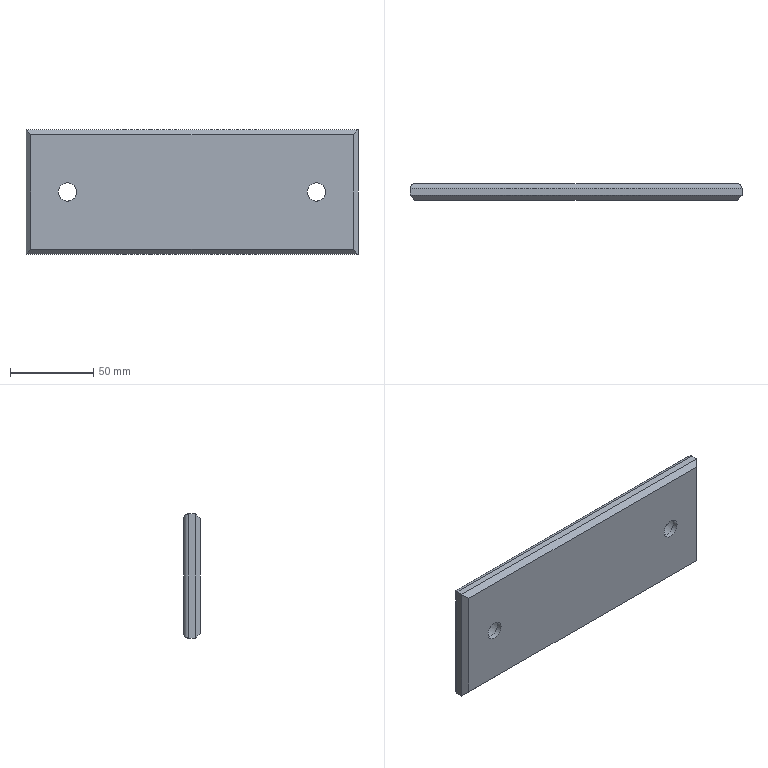Part | NX | features solid 2 | 1 solid | 20 faces | box 200 x 10 x 75 mm | volume 142571 mm3 | plane 12 | cylinder 8 | commonest cylinder face diameters 6 x4 11 x2 17.5 x2
STEP:
#1=CARTESIAN_POINT('',(-295.,288.,-290.));
#2=VERTEX_POINT('',#1);
#3=CARTESIAN_POINT('',(-295.,292.,-290.));
#4=VERTEX_POINT('',#3);
#5=CARTESIAN_POINT('',(-295.,285.,-290.));
#6=DIRECTION('',(0.,1.,0.));
#7=VECTOR('',#6,1000.);
#8=LINE('',#5,#7);
#9=EDGE_CURVE('',#2,#4,#8,.T.);
#10=ORIENTED_EDGE('',*,*,#9,.F.);
#11=CARTESIAN_POINT('',(-295.,288.,-365.));
#12=VERTEX_POINT('',#11);
#13=CARTESIAN_POINT('',(-295.,288.,-365.));
#14=DIRECTION('',(0.,0.,-1.));
#15=VECTOR('',#14,1000.);
#16=LINE('',#13,#15);
#17=EDGE_CURVE('',#2,#12,#16,.T.);
#18=ORIENTED_EDGE('',*,*,#17,.T.);
#19=CARTESIAN_POINT('',(-295.,292.,-365.));
#20=VERTEX_POINT('',#19);
#21=CARTESIAN_POINT('',(-295.,285.,-365.));
#22=DIRECTION('',(0.,1.,0.));
#23=VECTOR('',#22,1000.);
#24=LINE('',#21,#23);
#25=EDGE_CURVE('',#12,#20,#24,.T.);
#26=ORIENTED_EDGE('',*,*,#25,.T.);
#27=CARTESIAN_POINT('',(-295.,292.,-365.));
#28=DIRECTION('',(0.,0.,1.));
#29=VECTOR('',#28,1000.);
#30=LINE('',#27,#29);
#31=EDGE_CURVE('',#20,#4,#30,.T.);
#32=ORIENTED_EDGE('',*,*,#31,.T.);
#33=EDGE_LOOP('',(#10,#18,#26,#32));
#34=FACE_BOUND('',#33,.T.);
#35=CARTESIAN_POINT('',(-295.,285.,-365.));
#36=DIRECTION('',(-1.,0.,0.));
#37=DIRECTION('',(0.,1.,0.));
#38=AXIS2_PLACEMENT_3D('',#35,#36,#37);
#39=PLANE('',#38);
#40=ADVANCED_FACE('',(#34),#39,.F.);
#41=CARTESIAN_POINT('',(-495.,288.,-290.));
#42=VERTEX_POINT('',#41);
#43=CARTESIAN_POINT('',(-495.,292.,-290.));
#44=VERTEX_POINT('',#43);
#45=CARTESIAN_POINT('',(-495.,285.,-290.));
#46=DIRECTION('',(0.,1.,0.));
#47=VECTOR('',#46,1000.);
#48=LINE('',#45,#47);
#49=EDGE_CURVE('',#42,#44,#48,.T.);
#50=ORIENTED_EDGE('',*,*,#49,.F.);
#51=CARTESIAN_POINT('',(-295.,288.,-290.));
#52=DIRECTION('',(1.,0.,0.));
#53=VECTOR('',#52,1000.);
#54=LINE('',#51,#53);
#55=EDGE_CURVE('',#42,#2,#54,.T.);
#56=ORIENTED_EDGE('',*,*,#55,.T.);
#57=ORIENTED_EDGE('',*,*,#9,.T.);
#58=CARTESIAN_POINT('',(-295.,292.,-290.));
#59=DIRECTION('',(-1.,0.,0.));
#60=VECTOR('',#59,1000.);
#61=LINE('',#58,#60);
#62=EDGE_CURVE('',#4,#44,#61,.T.);
#63=ORIENTED_EDGE('',*,*,#62,.T.);
#64=EDGE_LOOP('',(#50,#56,#57,#63));
#65=FACE_BOUND('',#64,.T.);
#66=CARTESIAN_POINT('',(-295.,285.,-290.));
#67=DIRECTION('',(0.,0.,-1.));
#68=DIRECTION('',(0.,-1.,0.));
#69=AXIS2_PLACEMENT_3D('',#66,#67,#68);
#70=PLANE('',#69);
#71=ADVANCED_FACE('',(#65),#70,.F.);
#72=CARTESIAN_POINT('',(-495.,288.,-365.));
#73=VERTEX_POINT('',#72);
#74=CARTESIAN_POINT('',(-495.,292.,-365.));
#75=VERTEX_POINT('',#74);
#76=CARTESIAN_POINT('',(-495.,285.,-365.));
#77=DIRECTION('',(0.,1.,0.));
#78=VECTOR('',#77,1000.);
#79=LINE('',#76,#78);
#80=EDGE_CURVE('',#73,#75,#79,.T.);
#81=ORIENTED_EDGE('',*,*,#80,.F.);
#82=CARTESIAN_POINT('',(-495.,288.,-290.));
#83=DIRECTION('',(0.,0.,1.));
#84=VECTOR('',#83,1000.);
#85=LINE('',#82,#84);
#86=EDGE_CURVE('',#73,#42,#85,.T.);
#87=ORIENTED_EDGE('',*,*,#86,.T.);
#88=ORIENTED_EDGE('',*,*,#49,.T.);
#89=CARTESIAN_POINT('',(-495.,292.,-290.));
#90=DIRECTION('',(0.,0.,-1.));
#91=VECTOR('',#90,1000.);
#92=LINE('',#89,#91);
#93=EDGE_CURVE('',#44,#75,#92,.T.);
#94=ORIENTED_EDGE('',*,*,#93,.T.);
#95=EDGE_LOOP('',(#81,#87,#88,#94));
#96=FACE_BOUND('',#95,.T.);
#97=CARTESIAN_POINT('',(-495.,285.,-290.));
#98=DIRECTION('',(1.,0.,0.));
#99=DIRECTION('',(0.,-1.,0.));
#100=AXIS2_PLACEMENT_3D('',#97,#98,#99);
#101=PLANE('',#100);
#102=ADVANCED_FACE('',(#96),#101,.F.);
#103=ORIENTED_EDGE('',*,*,#25,.F.);
#104=CARTESIAN_POINT('',(-495.,288.,-365.));
#105=DIRECTION('',(-1.,0.,0.));
#106=VECTOR('',#105,1000.);
#107=LINE('',#104,#106);
#108=EDGE_CURVE('',#12,#73,#107,.T.);
#109=ORIENTED_EDGE('',*,*,#108,.T.);
#110=ORIENTED_EDGE('',*,*,#80,.T.);
#111=CARTESIAN_POINT('',(-495.,292.,-365.));
#112=DIRECTION('',(1.,0.,0.));
#113=VECTOR('',#112,1000.);
#114=LINE('',#111,#113);
#115=EDGE_CURVE('',#75,#20,#114,.T.);
#116=ORIENTED_EDGE('',*,*,#115,.T.);
#117=EDGE_LOOP('',(#103,#109,#110,#116));
#118=FACE_BOUND('',#117,.T.);
#119=CARTESIAN_POINT('',(-495.,285.,-365.));
#120=DIRECTION('',(0.,0.,1.));
#121=DIRECTION('',(-1.,0.,0.));
#122=AXIS2_PLACEMENT_3D('',#119,#120,#121);
#123=PLANE('',#122);
#124=ADVANCED_FACE('',(#118),#123,.F.);
#125=CARTESIAN_POINT('',(-298.,285.,-293.));
#126=VERTEX_POINT('',#125);
#127=CARTESIAN_POINT('',(-492.,285.,-293.));
#128=VERTEX_POINT('',#127);
#129=CARTESIAN_POINT('',(-495.,285.,-293.));
#130=DIRECTION('',(-1.,0.,0.));
#131=VECTOR('',#130,1000.);
#132=LINE('',#129,#131);
#133=EDGE_CURVE('',#126,#128,#132,.T.);
#134=ORIENTED_EDGE('',*,*,#133,.T.);
#135=CARTESIAN_POINT('',(-492.,285.,-362.));
#136=VERTEX_POINT('',#135);
#137=CARTESIAN_POINT('',(-492.,285.,-365.));
#138=DIRECTION('',(0.,0.,-1.));
#139=VECTOR('',#138,1000.);
#140=LINE('',#137,#139);
#141=EDGE_CURVE('',#128,#136,#140,.T.);
#142=ORIENTED_EDGE('',*,*,#141,.T.);
#143=CARTESIAN_POINT('',(-298.,285.,-362.));
#144=VERTEX_POINT('',#143);
#145=CARTESIAN_POINT('',(-295.,285.,-362.));
#146=DIRECTION('',(1.,0.,0.));
#147=VECTOR('',#146,1000.);
#148=LINE('',#145,#147);
#149=EDGE_CURVE('',#136,#144,#148,.T.);
#150=ORIENTED_EDGE('',*,*,#149,.T.);
#151=CARTESIAN_POINT('',(-298.,285.,-290.));
#152=DIRECTION('',(0.,0.,1.));
#153=VECTOR('',#152,1000.);
#154=LINE('',#151,#153);
#155=EDGE_CURVE('',#144,#126,#154,.T.);
#156=ORIENTED_EDGE('',*,*,#155,.T.);
#157=EDGE_LOOP('',(#134,#142,#150,#156));
#158=FACE_BOUND('',#157,.T.);
#159=CARTESIAN_POINT('',(-475.5,285.,-327.5));
#160=VERTEX_POINT('',#159);
#161=CARTESIAN_POINT('',(-470.,285.,-327.5));
#162=DIRECTION('',(0.,-1.,0.));
#163=DIRECTION('',(-1.,0.,0.));
#164=AXIS2_PLACEMENT_3D('',#161,#162,#163);
#165=CIRCLE('',#164,5.5);
#166=EDGE_CURVE('',#160,#160,#165,.T.);
#167=ORIENTED_EDGE('',*,*,#166,.F.);
#168=EDGE_LOOP('',(#167));
#169=FACE_BOUND('',#168,.T.);
#170=CARTESIAN_POINT('',(-325.5,285.,-327.5));
#171=VERTEX_POINT('',#170);
#172=CARTESIAN_POINT('',(-320.,285.,-327.5));
#173=DIRECTION('',(0.,-1.,0.));
#174=DIRECTION('',(-1.,0.,0.));
#175=AXIS2_PLACEMENT_3D('',#172,#173,#174);
#176=CIRCLE('',#175,5.5);
#177=EDGE_CURVE('',#171,#171,#176,.T.);
#178=ORIENTED_EDGE('',*,*,#177,.F.);
#179=EDGE_LOOP('',(#178));
#180=FACE_BOUND('',#179,.T.);
#181=CARTESIAN_POINT('',(-295.,285.,-290.));
#182=DIRECTION('',(0.,-1.,0.));
#183=DIRECTION('',(-1.,0.,0.));
#184=AXIS2_PLACEMENT_3D('',#181,#182,#183);
#185=PLANE('',#184);
#186=ADVANCED_FACE('',(#158,#169,#180),#185,.T.);
#187=CARTESIAN_POINT('',(-298.,295.,-293.));
#188=VERTEX_POINT('',#187);
#189=CARTESIAN_POINT('',(-298.,295.,-362.));
#190=VERTEX_POINT('',#189);
#191=CARTESIAN_POINT('',(-298.,295.,-290.));
#192=DIRECTION('',(0.,0.,1.));
#193=VECTOR('',#192,1000.);
#194=LINE('',#191,#193);
#195=EDGE_CURVE('',#188,#190,#194,.F.);
#196=ORIENTED_EDGE('',*,*,#195,.T.);
#197=CARTESIAN_POINT('',(-492.,295.,-362.));
#198=VERTEX_POINT('',#197);
#199=CARTESIAN_POINT('',(-295.,295.,-362.));
#200=DIRECTION('',(1.,0.,0.));
#201=VECTOR('',#200,1000.);
#202=LINE('',#199,#201);
#203=EDGE_CURVE('',#190,#198,#202,.F.);
#204=ORIENTED_EDGE('',*,*,#203,.T.);
#205=CARTESIAN_POINT('',(-492.,295.,-293.));
#206=VERTEX_POINT('',#205);
#207=CARTESIAN_POINT('',(-492.,295.,-290.));
#208=DIRECTION('',(0.,0.,-1.));
#209=VECTOR('',#208,1000.);
#210=LINE('',#207,#209);
#211=EDGE_CURVE('',#198,#206,#210,.F.);
#212=ORIENTED_EDGE('',*,*,#211,.T.);
#213=CARTESIAN_POINT('',(-295.,295.,-293.));
#214=DIRECTION('',(-1.,0.,0.));
#215=VECTOR('',#214,1000.);
#216=LINE('',#213,#215);
#217=EDGE_CURVE('',#206,#188,#216,.F.);
#218=ORIENTED_EDGE('',*,*,#217,.T.);
#219=EDGE_LOOP('',(#196,#204,#212,#218));
#220=FACE_BOUND('',#219,.T.);
#221=CARTESIAN_POINT('',(-478.75,295.,-327.5));
#222=VERTEX_POINT('',#221);
#223=CARTESIAN_POINT('',(-470.,295.,-327.5));
#224=DIRECTION('',(0.,-1.,0.));
#225=DIRECTION('',(-1.,0.,0.));
#226=AXIS2_PLACEMENT_3D('',#223,#224,#225);
#227=CIRCLE('',#226,8.75);
#228=EDGE_CURVE('',#222,#222,#227,.T.);
#229=ORIENTED_EDGE('',*,*,#228,.T.);
#230=EDGE_LOOP('',(#229));
#231=FACE_BOUND('',#230,.T.);
#232=CARTESIAN_POINT('',(-328.75,295.,-327.5));
#233=VERTEX_POINT('',#232);
#234=CARTESIAN_POINT('',(-320.,295.,-327.5));
#235=DIRECTION('',(0.,-1.,0.));
#236=DIRECTION('',(-1.,0.,0.));
#237=AXIS2_PLACEMENT_3D('',#234,#235,#236);
#238=CIRCLE('',#237,8.75);
#239=EDGE_CURVE('',#233,#233,#238,.T.);
#240=ORIENTED_EDGE('',*,*,#239,.T.);
#241=EDGE_LOOP('',(#240));
#242=FACE_BOUND('',#241,.T.);
#243=CARTESIAN_POINT('',(-295.,295.,-290.));
#244=DIRECTION('',(0.,-1.,0.));
#245=DIRECTION('',(-1.,0.,0.));
#246=AXIS2_PLACEMENT_3D('',#243,#244,#245);
#247=PLANE('',#246);
#248=ADVANCED_FACE('',(#220,#231,#242),#247,.F.);
#249=ORIENTED_EDGE('',*,*,#177,.T.);
#250=EDGE_LOOP('',(#249));
#251=FACE_BOUND('',#250,.T.);
#252=CARTESIAN_POINT('',(-320.,288.,-333.));
#253=VERTEX_POINT('',#252);
#254=CARTESIAN_POINT('',(-320.,288.,-327.5));
#255=DIRECTION('',(0.,-1.,0.));
#256=DIRECTION('',(0.,0.,-1.));
#257=AXIS2_PLACEMENT_3D('',#254,#255,#256);
#258=CIRCLE('',#257,5.5);
#259=EDGE_CURVE('',#253,#253,#258,.T.);
#260=ORIENTED_EDGE('',*,*,#259,.F.);
#261=EDGE_LOOP('',(#260));
#262=FACE_BOUND('',#261,.T.);
#263=CARTESIAN_POINT('',(-320.,255.,-327.5));
#264=DIRECTION('',(0.,-1.,0.));
#265=DIRECTION('',(-1.,0.,0.));
#266=AXIS2_PLACEMENT_3D('',#263,#264,#265);
#267=CYLINDRICAL_SURFACE('',#266,5.5);
#268=ADVANCED_FACE('',(#251,#262),#267,.F.);
#269=ORIENTED_EDGE('',*,*,#259,.T.);
#270=EDGE_LOOP('',(#269));
#271=FACE_BOUND('',#270,.T.);
#272=CARTESIAN_POINT('',(-320.,288.,-336.25));
#273=VERTEX_POINT('',#272);
#274=CARTESIAN_POINT('',(-320.,288.,-327.5));
#275=DIRECTION('',(0.,-1.,0.));
#276=DIRECTION('',(0.,0.,-1.));
#277=AXIS2_PLACEMENT_3D('',#274,#275,#276);
#278=CIRCLE('',#277,8.75);
#279=EDGE_CURVE('',#273,#273,#278,.T.);
#280=ORIENTED_EDGE('',*,*,#279,.F.);
#281=EDGE_LOOP('',(#280));
#282=FACE_BOUND('',#281,.T.);
#283=CARTESIAN_POINT('',(-320.,288.,-327.5));
#284=DIRECTION('',(0.,-1.,0.));
#285=DIRECTION('',(-1.,0.,0.));
#286=AXIS2_PLACEMENT_3D('',#283,#284,#285);
#287=PLANE('',#286);
#288=ADVANCED_FACE('',(#271,#282),#287,.F.);
#289=ORIENTED_EDGE('',*,*,#279,.T.);
#290=EDGE_LOOP('',(#289));
#291=FACE_BOUND('',#290,.T.);
#292=ORIENTED_EDGE('',*,*,#239,.F.);
#293=EDGE_LOOP('',(#292));
#294=FACE_BOUND('',#293,.T.);
#295=CARTESIAN_POINT('',(-320.,305.,-327.5));
#296=DIRECTION('',(0.,-1.,0.));
#297=DIRECTION('',(-1.,0.,0.));
#298=AXIS2_PLACEMENT_3D('',#295,#296,#297);
#299=CYLINDRICAL_SURFACE('',#298,8.75);
#300=ADVANCED_FACE('',(#291,#294),#299,.F.);
#301=ORIENTED_EDGE('',*,*,#166,.T.);
#302=EDGE_LOOP('',(#301));
#303=FACE_BOUND('',#302,.T.);
#304=CARTESIAN_POINT('',(-470.,288.,-333.));
#305=VERTEX_POINT('',#304);
#306=CARTESIAN_POINT('',(-470.,288.,-327.5));
#307=DIRECTION('',(0.,-1.,0.));
#308=DIRECTION('',(0.,0.,-1.));
#309=AXIS2_PLACEMENT_3D('',#306,#307,#308);
#310=CIRCLE('',#309,5.5);
#311=EDGE_CURVE('',#305,#305,#310,.T.);
#312=ORIENTED_EDGE('',*,*,#311,.F.);
#313=EDGE_LOOP('',(#312));
#314=FACE_BOUND('',#313,.T.);
#315=CARTESIAN_POINT('',(-470.,255.,-327.5));
#316=DIRECTION('',(0.,-1.,0.));
#317=DIRECTION('',(-1.,0.,0.));
#318=AXIS2_PLACEMENT_3D('',#315,#316,#317);
#319=CYLINDRICAL_SURFACE('',#318,5.5);
#320=ADVANCED_FACE('',(#303,#314),#319,.F.);
#321=ORIENTED_EDGE('',*,*,#311,.T.);
#322=EDGE_LOOP('',(#321));
#323=FACE_BOUND('',#322,.T.);
#324=CARTESIAN_POINT('',(-470.,288.,-336.25));
#325=VERTEX_POINT('',#324);
#326=CARTESIAN_POINT('',(-470.,288.,-327.5));
#327=DIRECTION('',(0.,-1.,0.));
#328=DIRECTION('',(0.,0.,-1.));
#329=AXIS2_PLACEMENT_3D('',#326,#327,#328);
#330=CIRCLE('',#329,8.75);
#331=EDGE_CURVE('',#325,#325,#330,.T.);
#332=ORIENTED_EDGE('',*,*,#331,.F.);
#333=EDGE_LOOP('',(#332));
#334=FACE_BOUND('',#333,.T.);
#335=CARTESIAN_POINT('',(-470.,288.,-327.5));
#336=DIRECTION('',(0.,-1.,0.));
#337=DIRECTION('',(-1.,0.,0.));
#338=AXIS2_PLACEMENT_3D('',#335,#336,#337);
#339=PLANE('',#338);
#340=ADVANCED_FACE('',(#323,#334),#339,.F.);
#341=ORIENTED_EDGE('',*,*,#331,.T.);
#342=EDGE_LOOP('',(#341));
#343=FACE_BOUND('',#342,.T.);
#344=ORIENTED_EDGE('',*,*,#228,.F.);
#345=EDGE_LOOP('',(#344));
#346=FACE_BOUND('',#345,.T.);
#347=CARTESIAN_POINT('',(-470.,305.,-327.5));
#348=DIRECTION('',(0.,-1.,0.));
#349=DIRECTION('',(-1.,0.,0.));
#350=AXIS2_PLACEMENT_3D('',#347,#348,#349);
#351=CYLINDRICAL_SURFACE('',#350,8.75);
#352=ADVANCED_FACE('',(#343,#346),#351,.F.);
#353=CARTESIAN_POINT('',(-298.,292.,-293.));
#354=DIRECTION('',(-0.7071,0.,0.7071));
#355=DIRECTION('',(0.7071,0.,0.7071));
#356=AXIS2_PLACEMENT_3D('',#353,#354,#355);
#357=ELLIPSE('',#356,4.243,3.);
#358=EDGE_CURVE('',#188,#4,#357,.F.);
#359=ORIENTED_EDGE('',*,*,#358,.F.);
#360=ORIENTED_EDGE('',*,*,#217,.F.);
#361=CARTESIAN_POINT('',(-492.,292.,-293.));
#362=DIRECTION('',(-0.7071,0.,-0.7071));
#363=DIRECTION('',(-0.7071,0.,0.7071));
#364=AXIS2_PLACEMENT_3D('',#361,#362,#363);
#365=ELLIPSE('',#364,4.243,3.);
#366=EDGE_CURVE('',#44,#206,#365,.T.);
#367=ORIENTED_EDGE('',*,*,#366,.F.);
#368=ORIENTED_EDGE('',*,*,#62,.F.);
#369=EDGE_LOOP('',(#359,#360,#367,#368));
#370=FACE_BOUND('',#369,.T.);
#371=CARTESIAN_POINT('',(-295.,292.,-293.));
#372=DIRECTION('',(-1.,0.,0.));
#373=DIRECTION('',(0.,1.,0.));
#374=AXIS2_PLACEMENT_3D('',#371,#372,#373);
#375=CYLINDRICAL_SURFACE('',#374,3.);
#376=ADVANCED_FACE('',(#370),#375,.T.);
#377=ORIENTED_EDGE('',*,*,#366,.T.);
#378=ORIENTED_EDGE('',*,*,#211,.F.);
#379=CARTESIAN_POINT('',(-492.,292.,-362.));
#380=DIRECTION('',(0.7071,0.,-0.7071));
#381=DIRECTION('',(-0.7071,0.,-0.7071));
#382=AXIS2_PLACEMENT_3D('',#379,#380,#381);
#383=ELLIPSE('',#382,4.243,3.);
#384=EDGE_CURVE('',#75,#198,#383,.T.);
#385=ORIENTED_EDGE('',*,*,#384,.F.);
#386=ORIENTED_EDGE('',*,*,#93,.F.);
#387=EDGE_LOOP('',(#377,#378,#385,#386));
#388=FACE_BOUND('',#387,.T.);
#389=CARTESIAN_POINT('',(-492.,292.,-290.));
#390=DIRECTION('',(0.,0.,-1.));
#391=DIRECTION('',(0.,-1.,0.));
#392=AXIS2_PLACEMENT_3D('',#389,#390,#391);
#393=CYLINDRICAL_SURFACE('',#392,3.);
#394=ADVANCED_FACE('',(#388),#393,.T.);
#395=ORIENTED_EDGE('',*,*,#358,.T.);
#396=ORIENTED_EDGE('',*,*,#31,.F.);
#397=CARTESIAN_POINT('',(-298.,292.,-362.));
#398=DIRECTION('',(0.7071,0.,0.7071));
#399=DIRECTION('',(-0.7071,0.,0.7071));
#400=AXIS2_PLACEMENT_3D('',#397,#398,#399);
#401=ELLIPSE('',#400,4.243,3.);
#402=EDGE_CURVE('',#190,#20,#401,.F.);
#403=ORIENTED_EDGE('',*,*,#402,.F.);
#404=ORIENTED_EDGE('',*,*,#195,.F.);
#405=EDGE_LOOP('',(#395,#396,#403,#404));
#406=FACE_BOUND('',#405,.T.);
#407=CARTESIAN_POINT('',(-298.,292.,-365.));
#408=DIRECTION('',(0.,0.,1.));
#409=DIRECTION('',(0.,1.,0.));
#410=AXIS2_PLACEMENT_3D('',#407,#408,#409);
#411=CYLINDRICAL_SURFACE('',#410,3.);
#412=ADVANCED_FACE('',(#406),#411,.T.);
#413=ORIENTED_EDGE('',*,*,#384,.T.);
#414=ORIENTED_EDGE('',*,*,#203,.F.);
#415=ORIENTED_EDGE('',*,*,#402,.T.);
#416=ORIENTED_EDGE('',*,*,#115,.F.);
#417=EDGE_LOOP('',(#413,#414,#415,#416));
#418=FACE_BOUND('',#417,.T.);
#419=CARTESIAN_POINT('',(-495.,292.,-362.));
#420=DIRECTION('',(1.,0.,0.));
#421=DIRECTION('',(0.,0.,1.));
#422=AXIS2_PLACEMENT_3D('',#419,#420,#421);
#423=CYLINDRICAL_SURFACE('',#422,3.);
#424=ADVANCED_FACE('',(#418),#423,.T.);
#425=CARTESIAN_POINT('',(-297.,286.,-363.));
#426=DIRECTION('',(-0.5774,-0.5774,0.5774));
#427=VECTOR('',#426,1000.);
#428=LINE('',#425,#427);
#429=EDGE_CURVE('',#12,#144,#428,.T.);
#430=ORIENTED_EDGE('',*,*,#429,.F.);
#431=ORIENTED_EDGE('',*,*,#17,.F.);
#432=CARTESIAN_POINT('',(-297.,286.,-292.));
#433=DIRECTION('',(-0.5774,-0.5774,-0.5774));
#434=VECTOR('',#433,1000.);
#435=LINE('',#432,#434);
#436=EDGE_CURVE('',#126,#2,#435,.F.);
#437=ORIENTED_EDGE('',*,*,#436,.F.);
#438=ORIENTED_EDGE('',*,*,#155,.F.);
#439=EDGE_LOOP('',(#430,#431,#437,#438));
#440=FACE_BOUND('',#439,.T.);
#441=CARTESIAN_POINT('',(-298.,285.,-290.));
#442=DIRECTION('',(0.7071,-0.7071,0.));
#443=DIRECTION('',(-0.7071,-0.7071,0.));
#444=AXIS2_PLACEMENT_3D('',#441,#442,#443);
#445=PLANE('',#444);
#446=ADVANCED_FACE('',(#440),#445,.T.);
#447=ORIENTED_EDGE('',*,*,#436,.T.);
#448=ORIENTED_EDGE('',*,*,#55,.F.);
#449=CARTESIAN_POINT('',(-426.333,219.333,-358.667));
#450=DIRECTION('',(0.5774,-0.5774,-0.5774));
#451=VECTOR('',#450,1000.);
#452=LINE('',#449,#451);
#453=EDGE_CURVE('',#128,#42,#452,.F.);
#454=ORIENTED_EDGE('',*,*,#453,.F.);
#455=ORIENTED_EDGE('',*,*,#133,.F.);
#456=EDGE_LOOP('',(#447,#448,#454,#455));
#457=FACE_BOUND('',#456,.T.);
#458=CARTESIAN_POINT('',(-295.,285.,-293.));
#459=DIRECTION('',(0.,-0.7071,0.7071));
#460=DIRECTION('',(0.,0.7071,0.7071));
#461=AXIS2_PLACEMENT_3D('',#458,#459,#460);
#462=PLANE('',#461);
#463=ADVANCED_FACE('',(#457),#462,.T.);
#464=ORIENTED_EDGE('',*,*,#429,.T.);
#465=ORIENTED_EDGE('',*,*,#149,.F.);
#466=CARTESIAN_POINT('',(-426.333,219.333,-296.333));
#467=DIRECTION('',(-0.5774,0.5774,-0.5774));
#468=VECTOR('',#467,1000.);
#469=LINE('',#466,#468);
#470=EDGE_CURVE('',#73,#136,#469,.F.);
#471=ORIENTED_EDGE('',*,*,#470,.F.);
#472=ORIENTED_EDGE('',*,*,#108,.F.);
#473=EDGE_LOOP('',(#464,#465,#471,#472));
#474=FACE_BOUND('',#473,.T.);
#475=CARTESIAN_POINT('',(-295.,285.,-362.));
#476=DIRECTION('',(0.,-0.7071,-0.7071));
#477=DIRECTION('',(0.,-0.7071,0.7071));
#478=AXIS2_PLACEMENT_3D('',#475,#476,#477);
#479=PLANE('',#478);
#480=ADVANCED_FACE('',(#474),#479,.T.);
#481=ORIENTED_EDGE('',*,*,#453,.T.);
#482=ORIENTED_EDGE('',*,*,#86,.F.);
#483=ORIENTED_EDGE('',*,*,#470,.T.);
#484=ORIENTED_EDGE('',*,*,#141,.F.);
#485=EDGE_LOOP('',(#481,#482,#483,#484));
#486=FACE_BOUND('',#485,.T.);
#487=CARTESIAN_POINT('',(-492.,285.,-290.));
#488=DIRECTION('',(-0.7071,-0.7071,0.));
#489=DIRECTION('',(-0.7071,0.7071,0.));
#490=AXIS2_PLACEMENT_3D('',#487,#488,#489);
#491=PLANE('',#490);
#492=ADVANCED_FACE('',(#486),#491,.T.);
#493=CLOSED_SHELL('',(#40,#71,#102,#124,#186,#248,#268,#288,#300,#320,#340,#352,#376,#394,#412,#424,#446,#463,#480,#492));
#494=MANIFOLD_SOLID_BREP('',#493);
#495=(LENGTH_UNIT()NAMED_UNIT(*)SI_UNIT(.MILLI.,.METRE.));
#496=UNCERTAINTY_MEASURE_WITH_UNIT(LENGTH_MEASURE(0.00001),#495,'','');
#497=(NAMED_UNIT(*)PLANE_ANGLE_UNIT()SI_UNIT($,.RADIAN.));
#498=(NAMED_UNIT(*)SI_UNIT($,.STERADIAN.)SOLID_ANGLE_UNIT());
#499=(GEOMETRIC_REPRESENTATION_CONTEXT(3)GLOBAL_UNCERTAINTY_ASSIGNED_CONTEXT((#496))GLOBAL_UNIT_ASSIGNED_CONTEXT((#495,#497,#498))REPRESENTATION_CONTEXT('',''));
#500=ADVANCED_BREP_SHAPE_REPRESENTATION('',(#494),#499);